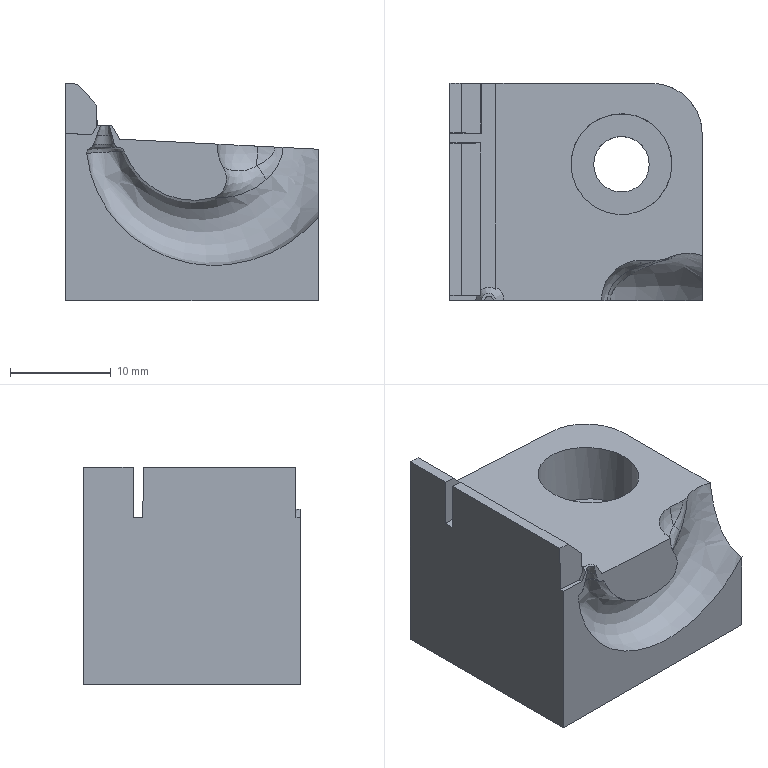Part | STEP file | solid 196 | 1 solid | 36 faces | box 25 x 21.5 x 21.524 mm | volume 7409 mm3 | plane 17 | spline 11 | cylinder 6 | cone 1 | sphere 1 | commonest cylinder face diameters 10 x2 6922 x2 5.5 x1 8 x1